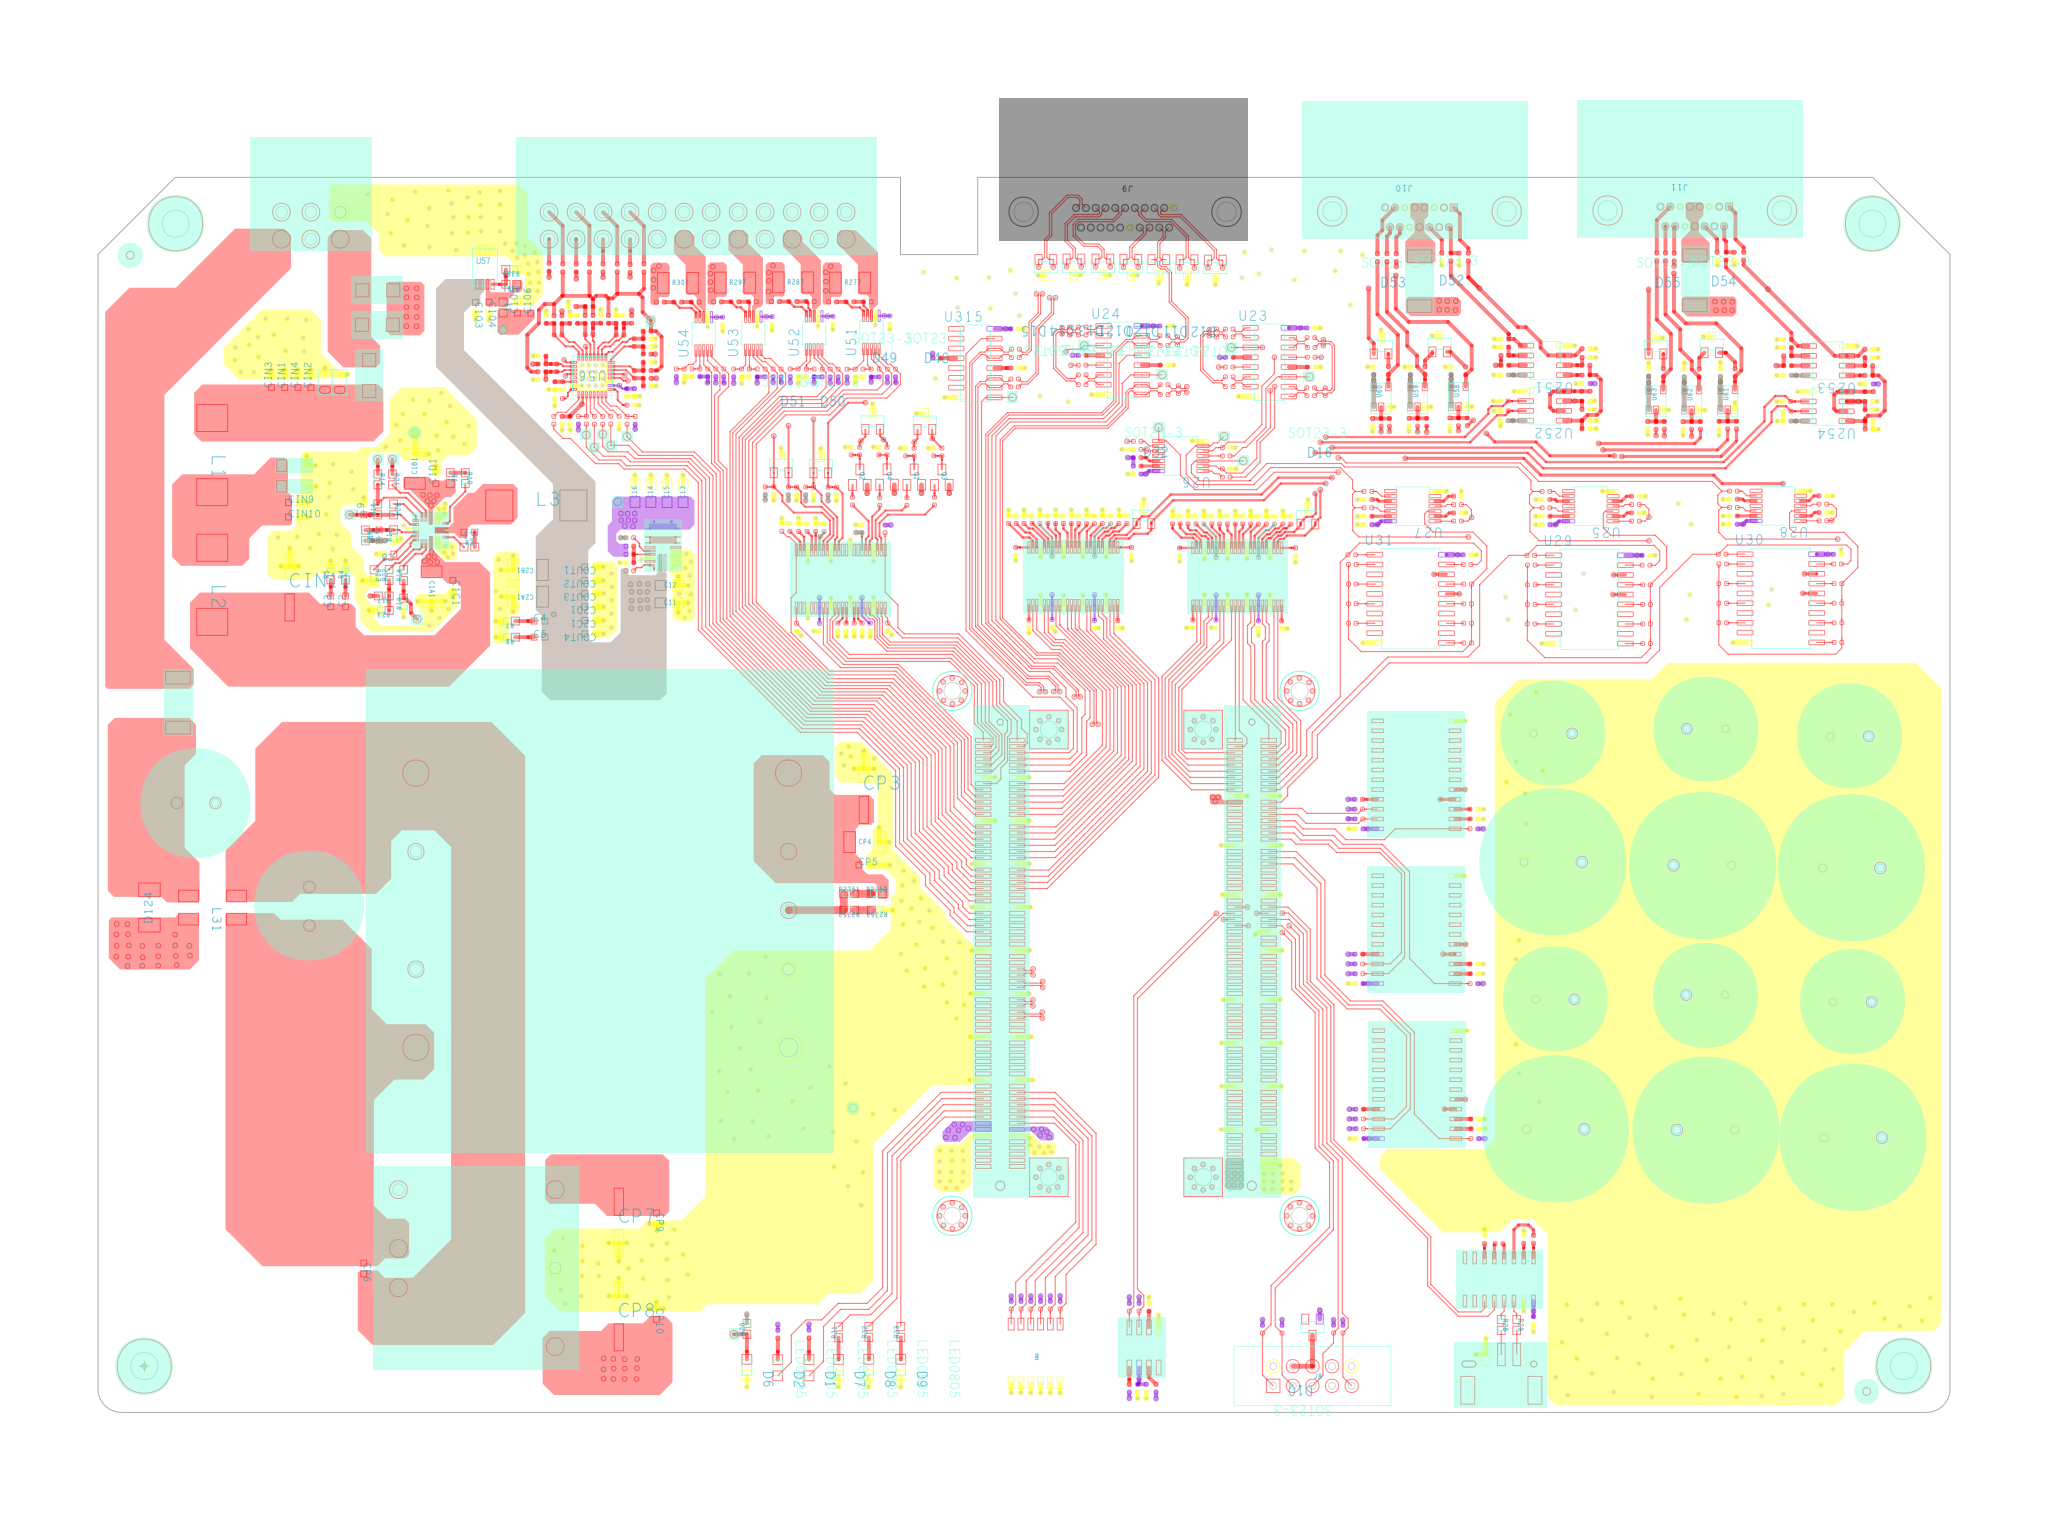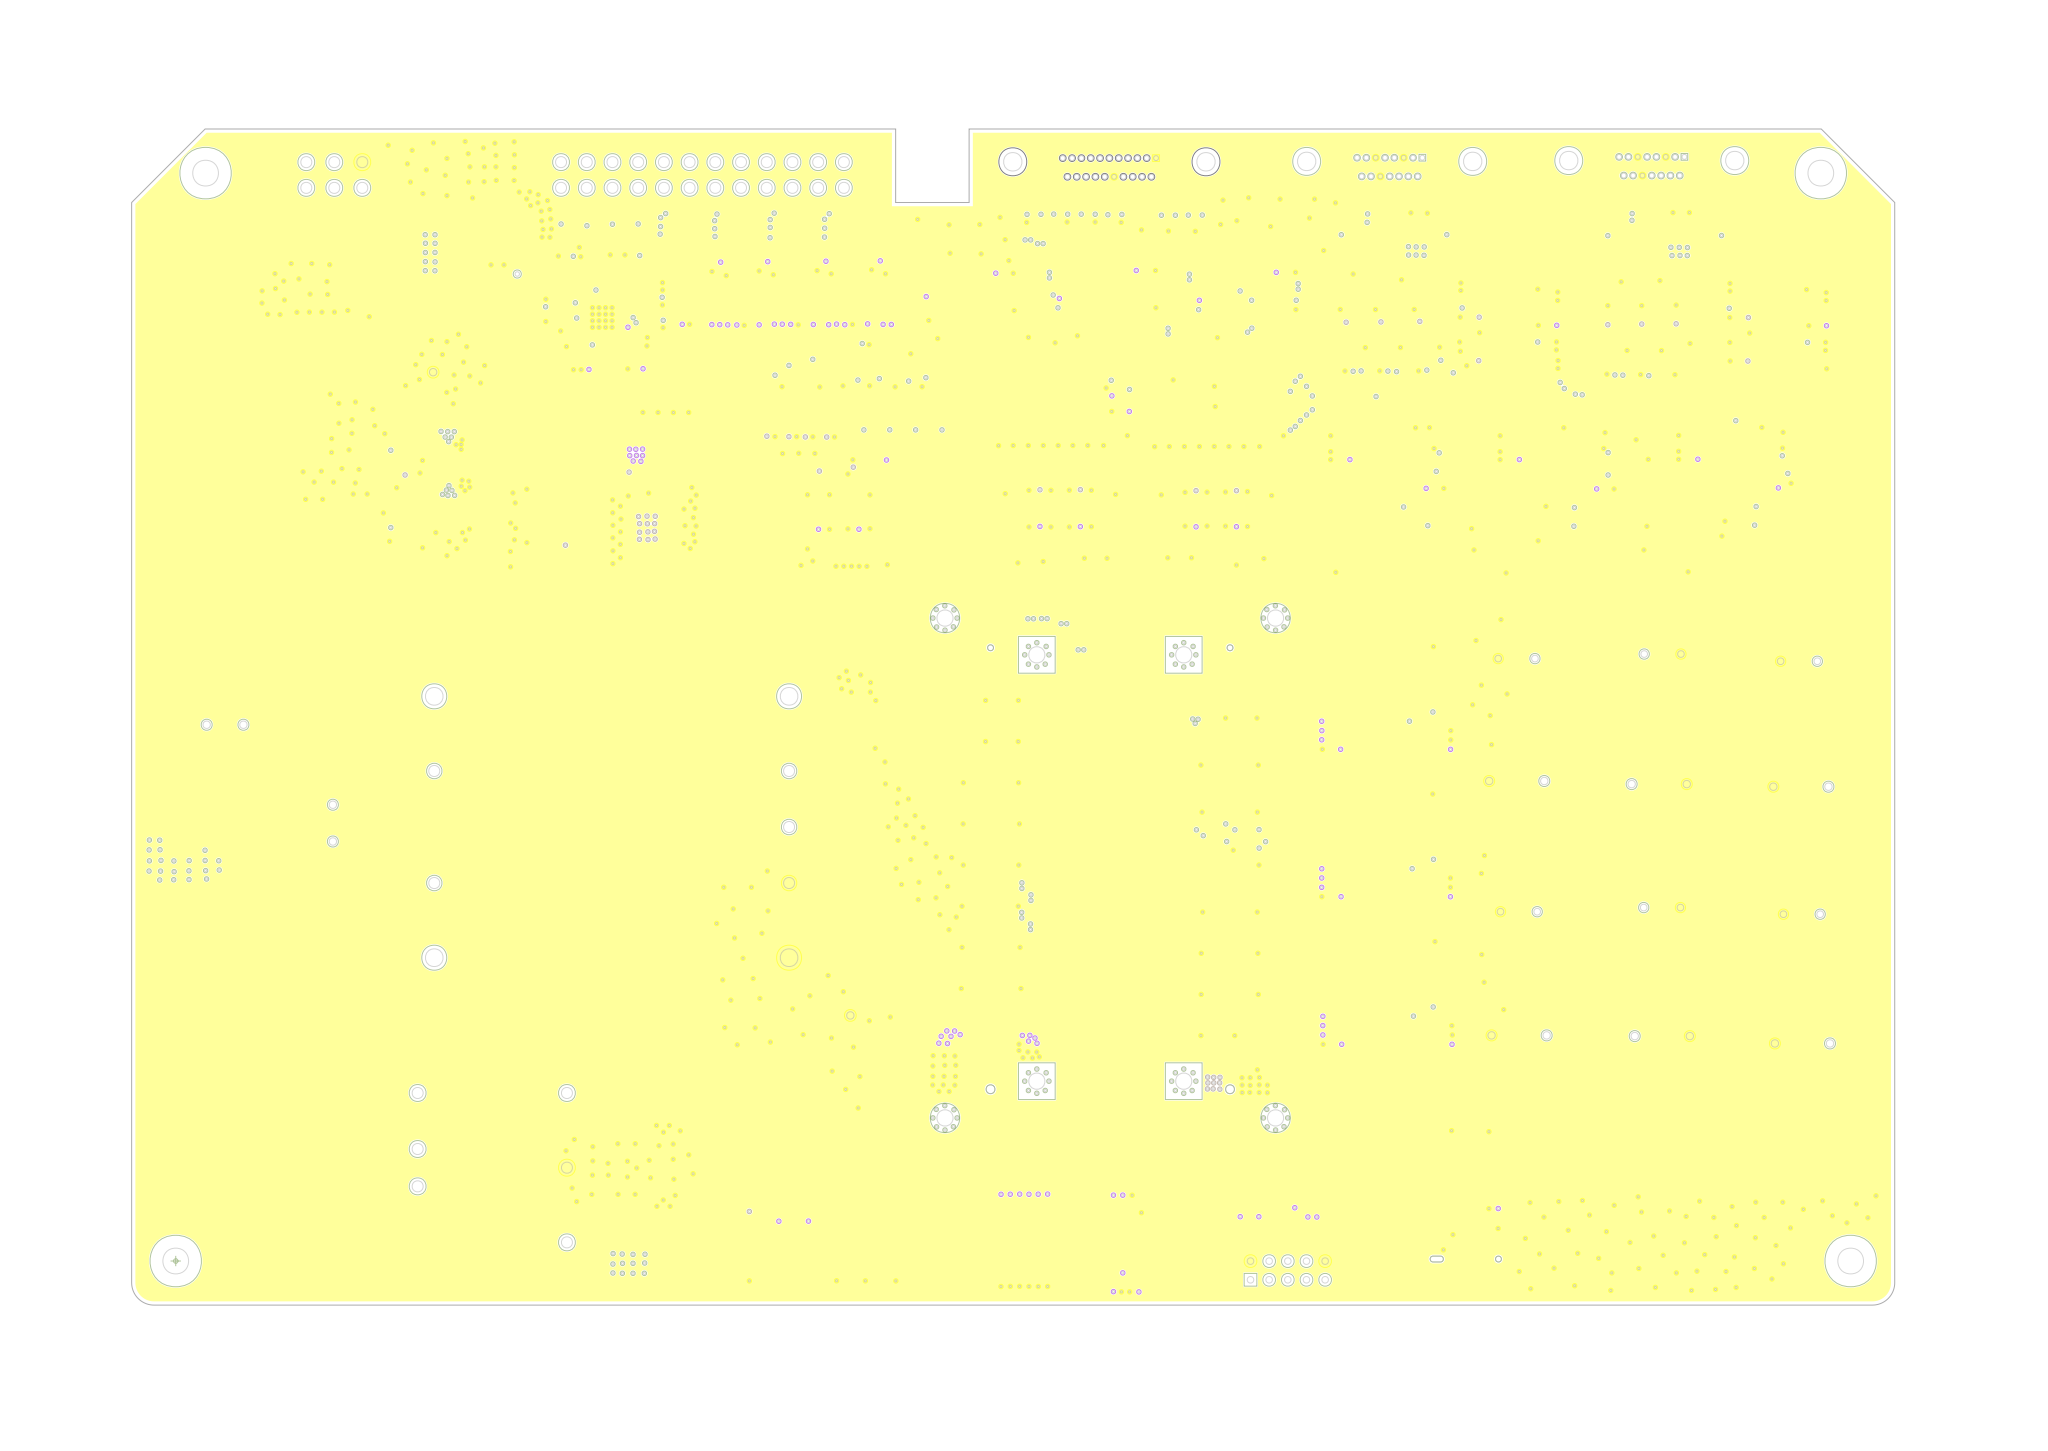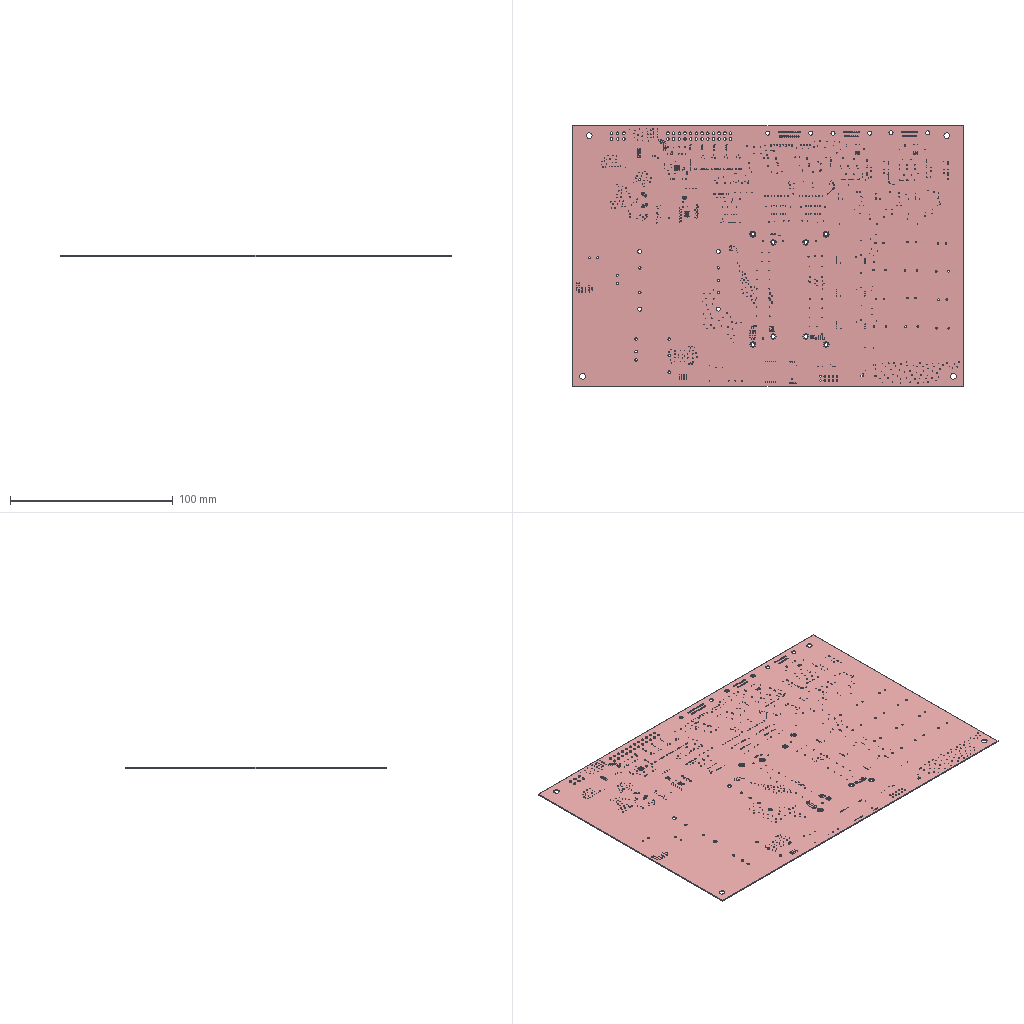Circuit board layout | Cadence Allegro | box 240 x 160 x 0.7 mm
Layer stack:
# Cadence Allegro layer stack of 2 (unit mm; from the constraint file cross-section; dielectric type: 0 not recorded (Allegro does not mark core vs prepreg), 3 surface material)
index,name,kind,layer,copper_thickness_mm,dielectric_type,dielectric_thickness_mm,dielectric_material,dielectric_constant
0,Top Surface,other,,,,,,
1,TOP,copper,TOP,0.0305,,,,
2,Dielectric1,dielectric,,,0,0.2032,FR-4,4.5
3,GND,copper,GND,0.0305,,,,
4,Dielectric2,dielectric,,,0,0.2032,FR-4,4.5
5,POWER,copper,POWER,0.0305,,,,
6,Dielectric3,dielectric,,,0,0.2032,FR-4,4.5
7,BOTTOM,copper,BOTTOM,0.0305,,,,
8,Bottom Surface,other,,,,,,
# drill layer pairs: low layer,high layer
drill_pair,TOP,BOTTOM
Part placement, first 399 of 635 lines:
REFDES,COMP_VALUE,SYM_NAME,SYM_X,SYM_Y,SYM_ROTATE,SYM_MIRROR
C1A1,CAP/1210,1210,1465.434,3976.499,270.000,NO
C1B1,CAP/1210,1210,1380.195,4577.161,90.000,NO
C1C1,CAP/0603,0603C,1574.039,4007.160,270.000,NO
C1D1,CAP/0603,0603C,1487.361,4501.515,90.000,NO
C2A1,CAP/1210,1210,1956.818,3924.329,180.000,NO
C2B1,CAP/1210,1210,1956.563,4060.550,180.000,NO
C2C1,CAP/0603,0603C,2303.126,3803.649,180.000,NO
C2D1,CAP/0603,0603C,2302.581,3873.143,180.000,NO
C1,CAP/0603,0603C,1685.688,4253.305,180.000,NO
C2,CAP/0603,0603C,1026.168,3873.029,90.000,NO
C3,CAP/0603,0603C,951.260,3873.232,90.000,NO
C4,CAP/0603,0603C,1988.129,3800.034,0.000,NO
C5,CAP/0603,0603C,1988.529,3717.881,0.000,NO
C6,CAP/0603,0603C,1198.333,4209.964,90.000,NO
C8,CAP/0603,0603C,1272.886,4141.786,180.000,NO
C9,CAP/0603,0603C,1120.158,4341.894,90.000,NO
C10,0.1uF/50V/10%/X7R/C0402,0402,7086.964,232.518,270.000,NO
C11,22uF/10V/10%/X5R/C0805,0805,2678.524,3892.734,0.000,NO
C12,22uF/10V/10%/X5R/C0805,0805,2678.800,3981.695,0.000,NO
C13,22uF/10V/10%/X5R/C0805,0805,2748.943,4451.876,90.000,NO
C14,22uF/10V/10%/X5R/C0805,0805,2584.754,4452.487,90.000,NO
C15,22uF/10V/10%/X5R/C0805,0805,2666.955,4451.762,90.000,NO
C16,22uF/10V/10%/X5R/C0805,0805,2503.522,4452.376,90.000,NO
C17,0.1uF/50V/10%/X7R/C0402,0402,7087.489,646.639,90.000,NO
C18,0.1uF/50V/10%/X7R/C0402,0402,6911.900,623.770,180.000,NO
C19,0.1uF/50V/10%/X7R/C0402,0402,7037.723,646.294,90.000,NO
C20,0.1uF/50V/10%/X7R/C0402,0402,6837.628,643.975,270.000,NO
C21,39pF/6.3V/5%/NP0/C0402,0402,2477.325,4140.263,180.000,NO
C22,1uF/16V/10%/X5R/C0402,0402,5068.182,-112.036,90.000,NO
C23,0.1uF/50V/10%/X7R/C0402,0402,5112.076,-112.284,90.000,NO
C24,0.1uF/50V/10%/X7R/C0402,0402,5125.671,299.907,90.000,NO
C25,0.1uF/50V/10%/X7R/C0402,0402,5951.524,5295.247,0.000,NO
C26,0.1uF/50V/10%/X7R/C0402,0402,5201.208,5305.263,0.000,NO
C27,0.1uF/50V/10%/X7R/C0402,0402,5065.955,4550.156,180.000,NO
C28,0.1uF/50V/10%/X7R/C0402,0402,7151.111,4291.950,180.000,NO
C29,0.1uF/50V/10%/X7R/C0402,0402,6242.994,4291.949,180.000,NO
C30,0.1uF/50V/10%/X7R/C0402,0402,8107.698,4293.779,180.000,NO
C31,0.1uF/50V/10%/X7R/C0402,0402,7660.842,4134.982,0.000,NO
C32,0.1uF/50V/10%/X7R/C0402,0402,6748.206,4138.240,0.000,NO
C33,0.1uF/50V/10%/X7R/C0402,0402,8637.483,4140.732,0.000,NO
C43,0.1uF/50V/10%/X7R/C0402,0402,6198.221,2740.667,0.000,NO
C45,0.1uF/50V/10%/X7R/C0402,0402,6198.573,1951.247,0.000,NO
C47,0.1uF/50V/10%/X7R/C0402,0402,6202.397,1160.643,0.000,NO
C49,0.1uF/50V/10%/X7R/C0402,0402,5766.891,4314.271,270.000,NO
C50,0.1uF/50V/10%/X7R/C0402,0402,5405.535,4315.049,270.000,NO
C51,0.1uF/50V/10%/X7R/C0402,0402,5467.835,3786.199,90.000,NO
C52,0.1uF/50V/10%/X7R/C0402,0402,5684.300,3781.656,90.000,NO
C57,0.1uF/50V/10%/X7R/C0402,0402,4930.365,4316.603,270.000,NO
C58,0.1uF/50V/10%/X7R/C0402,0402,4569.009,4317.381,270.000,NO
C59,0.1uF/50V/10%/X7R/C0402,0402,4847.774,3783.988,90.000,NO
C60,0.1uF/50V/10%/X7R/C0402,0402,4631.309,3788.531,90.000,NO
C65,0.1uF/50V/10%/X7R/C0402,0402,3803.741,5336.921,270.000,NO
C66,0.1uF/50V/10%/X7R/C0402,0402,3600.367,5428.470,0.000,NO
C67,0.1uF/50V/10%/X7R/C0402,0402,3512.888,5334.683,270.000,NO
C68,0.1uF/50V/10%/X7R/C0402,0402,3308.799,5429.878,0.000,NO
C69,0.1uF/50V/10%/X7R/C0402,0402,3202.484,5333.158,270.000,NO
C70,0.1uF/50V/10%/X7R/C0402,0402,3013.011,5428.470,0.000,NO
C71,0.1uF/50V/10%/X7R/C0402,0402,2950.344,5330.569,270.000,NO
C72,0.1uF/50V/10%/X7R/C0402,0402,2721.447,5427.062,0.000,NO
C73,0.1uF/50V/10%/X7R/C0402,0402,3661.662,4271.536,270.000,NO
C74,0.1uF/50V/10%/X7R/C0402,0402,3468.284,4276.953,270.000,NO
C75,0.1uF/50V/10%/X7R/C0402,0402,3444.743,3768.881,90.000,NO
C76,0.1uF/50V/10%/X7R/C0402,0402,3704.099,3770.174,90.000,NO
C77,10nF/50V/10%/X7R/C0402,0402,2565.299,4998.784,0.000,NO
C78,0.1uF/50V/10%/X7R/C0402,0402,2499.479,5058.201,90.000,NO
C79,10nF/50V/10%/X7R/C0402,0402,2565.078,5120.566,0.000,NO
C80,0.1uF/50V/10%/X7R/C0402,0402,2172.777,4824.301,270.000,NO
C81,1uF/50V/10%/X7R/C0402,0402,2131.567,4824.026,270.000,NO
C82,0.1uF/50V/10%/X7R/C0402,0402,2135.380,5001.091,270.000,NO
C83,1uF/50V/10%/X7R/C0402,0402,2094.388,5000.930,270.000,NO
C84,10nF/50V/10%/X7R/C0402,0402,2565.304,5200.458,0.000,NO
C85,0.1uF/50V/10%/X7R/C0402,0402,2497.547,5220.439,90.000,NO
C86,10nF/50V/10%/X7R/C0402,0402,2565.244,5240.239,0.000,NO
C87,0.1uF/50V/10%/X7R/C0402,0402,2113.766,4934.760,180.000,NO
C88,0.1uF/50V/10%/X7R/C0402,0402,2481.600,4901.211,0.000,NO
C89,0.1uF/50V/10%/X7R/C0402,0402,2460.040,4965.609,270.000,NO
C90,1uF/50V/10%/X7R/C0402,0402,2501.018,4966.074,270.000,NO
C91,10nF/50V/10%/X7R/C0402,0402,2446.425,5338.568,90.000,NO
C92,0.1uF/50V/10%/X7R/C0402,0402,2426.964,5258.168,180.000,NO
C93,10nF/50V/10%/X7R/C0402,0402,2407.207,5338.788,90.000,NO
C94,10nF/50V/10%/X7R/C0402,0402,2170.563,5338.047,90.000,NO
C95,0.1uF/50V/10%/X7R/C0402,0402,2110.730,5259.289,180.000,NO
C96,10nF/50V/10%/X7R/C0402,0402,2050.496,5337.941,90.000,NO
C99,10nF/50V/10%/X7R/C0402,0402,2029.187,5151.499,180.000,NO
C100,0.1uF/50V/10%/X7R/C0402,0402,2105.630,5091.446,270.000,NO
C101,10nF/50V/10%/X7R/C0402,0402,2028.852,5031.675,180.000,NO
C102,10nF/50V/10%/X7R/C0402,0402,2328.741,5338.869,90.000,NO
C103,1uF/25V/10%/X7R/C0603,0603C,1689.774,5424.503,270.000,NO
C104,1uF/25V/10%/X7R/C0603,0603C,1758.999,5426.586,270.000,NO
C105,10uF/10V/10%/X5R/C0603,0603C,1903.767,5370.918,90.000,NO
C106,0.1uF/50V/10%/X7R/C0603,0603C,1971.932,5370.859,90.000,NO
C107,0.1uF/50V/10%/X7R/C0402,0402,2269.120,5260.505,180.000,NO
C108,10nF/50V/10%/X7R/C0402,0402,2209.392,5338.368,90.000,NO
C109,0.1uF/50V/10%/X7R/C0402,0402,6666.908,5076.812,90.000,NO
C110,0.1uF/50V/10%/X7R/C0402,0402,6459.364,5076.456,90.000,NO
C111,0.1uF/50V/10%/X7R/C0402,0402,6272.476,5076.812,90.000,NO
C112,0.1uF/50V/10%/X7R/C0402,0402,8041.056,5066.436,90.000,NO
C113,0.1uF/50V/10%/X7R/C0402,0402,7674.891,5068.624,90.000,NO
C114,0.1uF/50V/10%/X7R/C0402,0402,7856.584,5065.004,90.000,NO
C795,0.1uF/50V/10%/X7R/C0402,0402,4439.984,5290.400,0.000,NO
C917,0.1uF/50V/10%/X7R/C0402,0402,6938.342,4822.335,180.000,NO
C918,2pF/50V/10%/X7R/C0402,0402,7354.384,4879.743,0.000,NO
C919,2pF/50V/10%/X7R/C0402,0402,7354.506,4822.784,0.000,NO
C920,0.1uF/50V/10%/X7R/C0402,0402,6940.936,5055.205,180.000,NO
C921,0.1uF/50V/10%/X7R/C0402,0402,8380.946,4820.319,180.000,NO
C922,0.1uF/50V/10%/X7R/C0402,0402,8383.540,5053.189,180.000,NO
C923,2pF/50V/10%/X7R/C0402,0402,8798.657,4877.394,0.000,NO
C924,2pF/50V/10%/X7R/C0402,0402,8799.113,4820.770,0.000,NO
C1046,10nF/50V/10%/X7R/C0402,0402,3211.543,4465.163,270.000,NO
C1047,10nF/50V/10%/X7R/C0402,0402,3414.415,4463.847,270.000,NO
C1048,10nF/50V/10%/X7R/C0402,0402,3327.631,4464.259,270.000,NO
C1049,10nF/50V/10%/X7R/C0402,0402,3530.643,4463.387,270.000,NO
CIN1,CAP/0603,0603C,716.126,4991.435,90.000,NO
CIN2,CAP/0603,0603C,850.372,4991.198,90.000,NO
CIN3,CAP/0603,0603C,649.394,4992.058,90.000,NO
CIN4,CAP/0603,0603C,783.533,4991.640,90.000,NO
CIN5,CAP/0603,0805C,921.995,5018.653,90.000,NO
CIN6,CAP/0603,0805C,996.502,5018.307,90.000,NO
CIN7,CAP/0603,1206,764.212,4593.485,0.000,NO
CIN8,CAP/0603,1206,763.877,4487.170,0.000,NO
CIN9,CAP/0603,0603C,735.616,4404.734,0.000,NO
CIN10,CAP/0603,0603C,735.616,4330.834,0.000,NO
CIN11,CAP/ELECT/DIP/OD5.3P2.0,AP-SMD_BD6_3-L6_6-W6_6-LS7_21,741.556,3974.623,90.000,NO
CIN12,ECF1HM182M27OTPO,AP-SMD_BD18-L27-W6_6-LS7_21,7186.624,2570.942,270.000,NO
CIN13,ECF1JM331G20OTPO,AP-SMD_BD10-L20-W6_6-LS7_21,7185.868,3226.632,270.000,NO
CIN14,ECF1HM182M27OTPO,AP-SMD_BD18-L27-W6_6-LS7_21,7199.516,1208.500,270.000,NO
CIN15,ECF1JM331G20OTPO,AP-SMD_BD10-L20-W6_6-LS7_21,7198.096,1870.916,270.000,NO
CIN16,ECF1HM182M27OTPO,AP-SMD_BD18-L27-W6_6-LS7_21,7966.783,1204.718,90.000,NO
CIN17,ECF1JM331G20OTPO,AP-SMD_BD10-L20-W6_6-LS7_21,7965.623,1893.086,90.000,NO
CIN18,ECF1HM182M27OTPO,AP-SMD_BD18-L27-W6_6-LS7_21,7950.310,2554.419,90.000,NO
CIN19,ECF1JM331G20OTPO,AP-SMD_BD10-L20-W6_6-LS7_21,7968.307,3250.966,90.000,NO
CIN20,ECF1HM182M27OTPO,AP-SMD_BD18-L27-W6_6-LS7_21,8709.621,2540.420,270.000,NO
CIN21,ECF1JM331G20OTPO,AP-SMD_BD10-L20-W6_6-LS7_21,8699.345,3212.322,270.000,NO
CIN22,ECF1HM182M27OTPO,AP-SMD_BD18-L27-W6_6-LS7_21,8717.937,1165.386,270.000,NO
CIN23,ECF1JM331G20OTPO,AP-SMD_BD10-L20-W6_6-LS7_21,8714.565,1857.490,270.000,NO
COUT1,CAP/0603,0603C,2302.361,4076.388,180.000,NO
COUT2,CAP/0603,0603C,2302.286,4007.628,180.000,NO
COUT3,CAP/0603,0603C,2302.924,3940.616,180.000,NO
COUT4,CAP/0603,0603C,2303.728,3735.215,180.000,NO
CP1,CAP/ELECT/DIP/OD5.3P2.0,AP-SMD_BD12_5-L20,264.324,2872.264,0.000,NO
CP2,CAP/ELECT/DIP/OD5.3P2.0,AP-SMD_BD12_5-L20,842.187,2345.380,270.000,NO
CP3,CAP/ELECT/DIP/OD5.3P2.0,AP-SMD_BD6_3-L6_6-W6_6-LS7_21,3670.733,2941.914,90.000,NO
CP4,CAP/1210,1210,3673.410,2672.756,0.000,NO
CP5,CAP/0603,0603C,3645.741,2555.662,0.000,NO
CP6,CAP/0603,0603C,1119.792,525.680,270.000,NO
CP7,CAP/ELECT/DIP/OD5.3P2.0,AP-SMD_BD6_3-L6_6-W6_6-LS7_21,2420.880,733.340,90.000,NO
CP8,CAP/ELECT/DIP/OD5.3P2.0,AP-SMD_BD6_3-L6_6-W6_6-LS7_21,2420.880,252.164,90.000,NO
CP9,CAP/0603,0603C,2613.744,781.072,270.000,NO
CP10,CAP/0603,0603C,2612.768,293.072,270.000,NO
D1,LED_GREEN,LED0805,3391.153,-8.170,270.000,NO
D2,LED_GREEN,LED0805,3231.645,-8.055,270.000,NO
D3,SS34,DO-214AC,1147.161,5052.210,270.000,NO
D6,LED_GREEN,LED0805,3074.152,-6.494,270.000,NO
D7,LED_GREEN,LED0805,3541.603,-6.906,270.000,NO
D8,LED_GREEN,LED0805,3695.910,-6.451,270.000,NO
D9,LED_GREEN,LED0805,3859.228,-6.536,270.000,NO
D10,BAT54C,SOT23,5959.891,198.860,180.000,NO
D11,PESD5V0L2BT,SOT23,5319.914,5602.014,180.000,NO
D12,PESD5V0L2BT,SOT23,5464.066,5600.018,180.000,NO
D13,PESD5V0L2BT,SOT23,4890.281,5605.666,180.000,NO
D14,PESD5V0L2BT,SOT23,4742.737,5605.666,180.000,NO
D15,PESD5V0L2BT,SOT23,4599.667,5603.752,180.000,NO
D16,PESD5V0L2BT,SOT23,5936.588,4335.974,0.000,NO
D32,PESD5V0L2BT,SOT23,5100.062,4338.306,0.000,NO
D48,PESD5V0L2BT,SOT23,3982.229,4818.243,0.000,NO
D49,PESD5V0L2BT,SOT23,3715.947,4818.975,0.000,NO
D50,PESD5V0L2BT,SOT23,3451.439,4596.863,0.000,NO
D51,PESD5V0L2BT,SOT23,3249.068,4597.791,0.000,NO
D52,PESD5V0L2BT,SOT23,6608.828,5214.298,0.000,NO
D53,PESD5V0L2BT,SOT23,6310.029,5203.769,0.000,NO
D54,PESD5V0L2BT,SOT23,7996.840,5209.814,0.000,NO
D55,PESD5V0L2BT,SOT23,7712.440,5203.528,0.000,NO
D120,PESD5V0L2BT,SOT23,5175.702,5602.685,180.000,NO
D121,PESD5V0L2BT,SOT23,5033.114,5603.965,180.000,NO
D122,SS34,DO-214AC,1189.269,5311.224,0.000,NO
D123,SS34,DO-214AC,1191.063,5487.208,0.000,NO
D124,SM6T56AY,DO-214AA,26.179,2339.032,90.000,NO
E1,Inductor_BEAD,0603R,1830.290,5399.204,270.000,NO
E14,Inductor_BEAD,0603R,1882.173,5925.017,0.000,YES
E15,Inductor_BEAD,0603R,1882.536,5994.352,0.000,YES
E16,Inductor_BEAD,0603R,1882.028,5856.252,0.000,YES
E17,Inductor_BEAD,0603R,1881.520,5787.460,0.000,YES
F1,0451010.MRL 125V@10A 2512,2512,171.492,3383.936,270.000,NO
J1,D2_3,D2_3,4614.756,3246.749,180.000,NO
J2,D2_3,D2_3,5402.154,3246.749,180.000,NO
J3,D2_3,D2_3,5402.154,963.280,180.000,NO
J4,D2_3,D2_3,4614.756,963.280,180.000,NO
J7,BM03B-PASS,BM03B-PASS,6923.507,59.754,0.000,NO
J8,TC2050_IDC_FP1,JTAG-10,5759.948,-100.535,0.000,NO
J9,J30JA-21ZKW-J,J30JA-21ZKW-J,5003.698,5887.469,180.000,NO
J10,J30JA-15ZKW-J,J30JA-15ZKW-J,6505.872,5889.544,180.000,NO
J11,J30JA-15ZKW-J,J30JA-15ZKW-J,7910.384,5894.004,180.000,NO
JX1,5177984-6,5177983-6,4366.721,2105.016,90.000,NO
JX2,5177984-6,5177983-6,5650.185,2105.016,90.000,NO
L1,CKST1004-1uH/M-B,SMD_10X11,346.314,4646.925,270.000,NO
L2,CKST1004-4.7uH/M,SMD_10X11,346.216,3984.972,270.000,NO
L3,CKST1004-4.7uH/M,SMD_10X11,2000.176,4389.846,0.000,NO
L31,YLM1513-701T,SMD_7X6MM,348.247,2338.740,270.000,NO
P1,F83-S-3.5-24pin,F83-S-3_5-24PIN,2822.870,5747.949,180.000,NO
P2,F83-S-3.81-6pin,F83-S-3_81-6PIN,849.744,5747.796,180.000,NO
Q1,S8050,SOT-23,3927.779,4533.749,270.000,NO
Q2,S8050,SOT-23,3650.422,4533.537,270.000,NO
Q3,S8050,SOT-23,4068.992,4533.332,270.000,NO
Q4,S8050,SOT-23,3789.052,4534.430,270.000,NO
R1,1K/62.5mW/1%/R0402,0402,3391.000,163.952,90.000,NO
R2,1K/62.5mW/1%/R0402,0402,3232.228,162.889,90.000,NO
R3,0/62.5mW/1%/R0603,0603R,1658.428,4177.456,0.000,NO
R4,10/62.5mW/1%/R0603,0603R,1026.009,4037.430,90.000,NO
R5,10/62.5mW/1%/R0603,0603R,951.264,4037.890,90.000,NO
R6,100K/62.5mW/1%/R0603,0603R,1560.839,4529.069,270.000,NO
R7,10/62.5mW/1%/R0603,0603R,1865.289,3800.193,180.000,NO
R8,10/62.5mW/1%/R0603,0603R,1865.325,3717.964,180.000,NO
R9,100K/62.5mW/1%/R0603,0603R,1128.152,4237.129,270.000,NO
R10,10/62.5mW/1%/R0603,0603R,1637.704,4528.939,270.000,NO
R12,19.6K/62.5mW/1%/R0603,0603R,1271.488,4237.678,90.000,NO
R13,62K/62.5mW/1%/R0603,0603R,1172.144,4034.230,270.000,NO
R14,10/62.5mW/1%/R0603,0603R,1191.305,4522.327,270.000,NO
R16,100K/62.5mW/1%/R0603,0603R,1190.815,4369.467,90.000,NO
R17,10/62.5mW/1%/R0603,0603R,1221.396,3928.232,180.000,NO
R18,10/62.5mW/1%/R0603,0603R,1322.955,4033.851,90.000,NO
R19,51K/62.5mW/1%/R0603,0603R,1322.916,3889.450,90.000,NO
R20,10K/62.5mW/1%/R0603,0603R,3074.090,189.923,90.000,NO
R21,10/62.5mW/1%/R0603,0603R,1265.684,4522.258,270.000,NO
R22,10/62.5mW/1%/R0603,0603R,1248.944,4035.206,90.000,NO
R23,0/62.5mW/1%/R0603,0603R,1221.711,3854.492,180.000,NO
R24,10/62.5mW/1%/R0603,0603R,1271.829,4369.506,270.000,NO
R25,499K/62.5mW/1%/R0402,0402,2476.720,4225.317,0.000,NO
R26,100k/62.5mW/1%/R0402,0402,2476.831,4056.949,180.000,NO
R27,20K/62.5mW/1%/R0402,0402,2477.212,4182.388,0.000,NO
R28,10/62.5mW/1%/R0603,0603R,6923.022,209.802,270.000,NO
R29,10/62.5mW/1%/R0603,0603R,7001.660,210.715,270.000,NO
R30,4.42K/62.5mW/1%/R0402,0402,2477.244,4097.576,0.000,NO
R31,10K/62.5mW/1%/R0603,0603R,3541.781,172.441,90.000,NO
R32,10K/62.5mW/1%/R0603,0603R,3696.642,174.411,90.000,NO
R33,10K/62.5mW/1%/R0603,0603R,3859.751,174.562,90.000,NO
R34,10K/62.5mW/1%/R0402,0402,4422.937,310.839,270.000,NO
R35,10K/62.5mW/1%/R0402,0402,4472.476,310.950,270.000,NO
R36,10K/62.5mW/1%/R0402,0402,4522.917,310.520,270.000,NO
R37,10K/62.5mW/1%/R0402,0402,4572.645,310.513,270.000,NO
R38,10K/62.5mW/1%/R0402,0402,4622.134,310.953,270.000,NO
R39,10K/62.5mW/1%/R0402,0402,4672.740,310.678,270.000,NO
R40,4.7K/62.5mW/1%/R0402,0402,5704.804,188.504,270.000,NO
R41,4.7K/62.5mW/1%/R0402,0402,5804.612,188.432,270.000,NO
R42,4.7K/62.5mW/1%/R0402,0402,6067.480,189.176,270.000,NO
R43,4.7K/62.5mW/1%/R0402,0402,6115.248,188.844,270.000,NO
R44,4.7K/62.5mW/1%/R0402,0402,5161.812,-112.620,90.000,NO
R45,4.7K/62.5mW/1%/R0402,0402,5025.475,-113.306,90.000,NO
R46,4.7K/62.5mW/1%/R0402,0402,5025.425,300.205,270.000,NO
R47,4.7K/62.5mW/1%/R0402,0402,5075.349,300.222,270.000,NO
R48,22/62.5mW/1%/R0402,0402,5953.854,5095.751,0.000,NO
R49,0/62.5mW/1%/R0402,0402,5535.386,5249.841,0.000,NO
R50,0/62.5mW/1%/R0402,0402,5535.292,5288.963,0.000,NO
R51,22/62.5mW/1%/R0402,0402,5203.538,5105.767,0.000,NO
R52,0/62.5mW/1%/R0402,0402,5535.379,5045.522,0.000,NO
R53,0/62.5mW/1%/R0402,0402,4785.070,5259.857,0.000,NO
R54,0/62.5mW/1%/R0402,0402,4784.976,5298.979,0.000,NO
R55,0/62.5mW/1%/R0402,0402,5535.158,4995.824,0.000,NO
R56,0/62.5mW/1%/R0402,0402,4785.063,5055.538,0.000,NO
R57,0/62.5mW/1%/R0402,0402,5950.603,4989.357,180.000,NO
R58,0/62.5mW/1%/R0402,0402,4784.842,5005.840,0.000,NO
R59,10K/62.5mW/1%/R0402,0402,5535.949,5145.458,0.000,NO
R60,0/62.5mW/1%/R0402,0402,5951.166,4949.684,180.000,NO
R61,0/62.5mW/1%/R0402,0402,5953.217,5195.503,180.000,NO
R62,10K/62.5mW/1%/R0402,0402,4785.633,5155.474,0.000,NO
R63,0/62.5mW/1%/R0402,0402,5952.107,5245.526,180.000,NO
R64,0/62.5mW/1%/R0402,0402,5202.994,5005.686,180.000,NO
R65,0/62.5mW/1%/R0402,0402,5203.290,4955.649,180.000,NO
R66,0/62.5mW/1%/R0402,0402,5202.901,5205.519,180.000,NO
R67,0/62.5mW/1%/R0402,0402,5201.791,5255.542,180.000,NO
R68,0/62.5mW/1%/R0402,0402,5519.910,4534.523,180.000,NO
R69,0/62.5mW/1%/R0402,0402,7607.919,4309.953,180.000,NO
R70,0/62.5mW/1%/R0402,0402,7607.612,4394.296,180.000,NO
R71,1k/62.5mW/1%/R0402,0402,5519.800,4576.523,180.000,NO
R72,0/62.5mW/1%/R0402,0402,5519.831,4642.186,180.000,NO
R73,0/62.5mW/1%/R0402,0402,6699.802,4309.952,180.000,NO
R74,0/62.5mW/1%/R0402,0402,6699.495,4394.295,180.000,NO
R75,0/62.5mW/1%/R0402,0402,8564.506,4311.782,180.000,NO
R76,0/62.5mW/1%/R0402,0402,7607.809,4351.953,180.000,NO
R77,0/62.5mW/1%/R0402,0402,6699.692,4351.952,180.000,NO
R78,0/62.5mW/1%/R0402,0402,8564.199,4396.125,180.000,NO
R79,0/62.5mW/1%/R0402,0402,8564.396,4353.782,180.000,NO
R80,1k/62.5mW/1%/R0402,0402,5519.709,4684.753,180.000,NO
R81,0/62.5mW/1%/R0402,0402,7607.490,4436.863,180.000,NO
R82,0/62.5mW/1%/R0402,0402,6699.373,4436.862,180.000,NO
R83,0/62.5mW/1%/R0402,0402,8564.077,4438.692,180.000,NO
R84,0/62.5mW/1%/R0402,0402,5065.540,4717.116,0.000,NO
R85,0/62.5mW/1%/R0402,0402,7151.067,4461.202,0.000,NO
R86,0/62.5mW/1%/R0402,0402,6242.950,4461.201,0.000,NO
R87,0/62.5mW/1%/R0402,0402,8107.654,4463.031,0.000,NO
R88,1k/62.5mW/1%/R0402,0402,5065.702,4675.955,0.000,NO
R89,0/62.5mW/1%/R0402,0402,7151.229,4420.040,0.000,NO
R90,0/62.5mW/1%/R0402,0402,6243.112,4420.039,0.000,NO
R91,0/62.5mW/1%/R0402,0402,8107.816,4421.869,0.000,NO
R92,1k/62.5mW/1%/R0402,0402,5065.501,4633.754,0.000,NO
R93,0/62.5mW/1%/R0402,0402,7151.028,4377.840,0.000,NO
R94,0/62.5mW/1%/R0402,0402,6242.911,4377.839,0.000,NO
R95,0/62.5mW/1%/R0402,0402,8107.615,4379.669,0.000,NO
R96,1k/62.5mW/1%/R0402,0402,5065.662,4590.620,0.000,NO
R97,0/62.5mW/1%/R0402,0402,7151.189,4334.706,0.000,NO
R98,0/62.5mW/1%/R0402,0402,6243.072,4334.705,0.000,NO
R99,0/62.5mW/1%/R0402,0402,8107.776,4336.535,0.000,NO
R100,0/62.5mW/1%/R0402,0402,7076.219,4085.572,0.000,NO
R101,0/62.5mW/1%/R0402,0402,6163.583,4088.830,0.000,NO
R102,0/62.5mW/1%/R0402,0402,8052.860,4091.322,0.000,NO
R103,0/62.5mW/1%/R0402,0402,7076.141,3985.465,0.000,NO
R104,0/62.5mW/1%/R0402,0402,7075.987,3885.370,0.000,NO
R105,0/62.5mW/1%/R0402,0402,6163.505,3988.723,0.000,NO
R106,0/62.5mW/1%/R0402,0402,8052.628,3891.120,0.000,NO
R107,0/62.5mW/1%/R0402,0402,6163.217,3788.924,0.000,NO
R108,0/62.5mW/1%/R0402,0402,6163.351,3888.628,0.000,NO
R109,0/62.5mW/1%/R0402,0402,7075.853,3785.666,0.000,NO
R110,0/62.5mW/1%/R0402,0402,8052.782,3991.215,0.000,NO
R111,0/62.5mW/1%/R0402,0402,8052.494,3791.416,0.000,NO
R112,0/62.5mW/1%/R0402,0402,7664.139,3685.691,180.000,NO
R113,0/62.5mW/1%/R0402,0402,6751.503,3688.491,180.000,NO
R114,0/62.5mW/1%/R0402,0402,8640.780,3691.057,180.000,NO
R115,0/62.5mW/1%/R0402,0402,7664.395,3785.755,180.000,NO
R116,0/62.5mW/1%/R0402,0402,6751.759,3789.013,180.000,NO
R117,0/62.5mW/1%/R0402,0402,8641.036,3791.301,180.000,NO
R118,0/62.5mW/1%/R0402,0402,7663.976,3885.181,180.000,NO
R119,0/62.5mW/1%/R0402,0402,6751.340,3888.439,180.000,NO
R120,0/62.5mW/1%/R0402,0402,8640.719,3891.135,180.000,NO
R121,0/62.5mW/1%/R0402,0402,7664.109,3985.288,180.000,NO
R122,0/62.5mW/1%/R0402,0402,6751.473,3988.546,180.000,NO
R123,0/62.5mW/1%/R0402,0402,8640.750,3991.140,180.000,NO
R124,0/62.5mW/1%/R0402,0402,7661.573,4085.193,180.000,NO
R125,0/62.5mW/1%/R0402,0402,6748.937,4088.451,180.000,NO
R126,0/62.5mW/1%/R0402,0402,8638.214,4091.147,180.000,NO
R127,0/62.5mW/1%/R0402,0402,7073.447,4135.209,0.000,NO
R128,0/62.5mW/1%/R0402,0402,6160.811,4138.467,0.000,NO
R129,0/62.5mW/1%/R0402,0402,8050.088,4140.959,0.000,NO
R220,10K/62.5mW/1%/R0402,0402,6195.676,2890.858,0.000,NO
R221,10K/62.5mW/1%/R0402,0402,6784.445,2790.804,180.000,NO
R222,10K/62.5mW/1%/R0402,0402,6783.181,2840.724,180.000,NO
R226,10K/62.5mW/1%/R0402,0402,6783.382,2740.450,0.000,NO
R228,10K/62.5mW/1%/R0402,0402,6195.866,2840.911,180.000,NO
R230,10K/62.5mW/1%/R0402,0402,6197.177,2790.860,180.000,NO
R232,10K/62.5mW/1%/R0402,0402,6196.232,2101.029,0.000,NO
R233,10K/62.5mW/1%/R0402,0402,6784.797,2001.384,180.000,NO
R234,10K/62.5mW/1%/R0402,0402,6783.533,2051.304,180.000,NO
R238,10K/62.5mW/1%/R0402,0402,6783.734,1951.030,0.000,NO
R240,10K/62.5mW/1%/R0402,0402,6196.218,2051.491,180.000,NO
R242,10K/62.5mW/1%/R0402,0402,6197.529,2001.440,180.000,NO
R244,10K/62.5mW/1%/R0402,0402,6200.056,1310.425,0.000,NO
R245,10K/62.5mW/1%/R0402,0402,6788.621,1210.780,180.000,NO
R246,10K/62.5mW/1%/R0402,0402,6787.357,1260.700,180.000,NO
R250,10K/62.5mW/1%/R0402,0402,6787.558,1160.426,0.000,NO
R252,10K/62.5mW/1%/R0402,0402,6200.042,1260.887,180.000,NO
R254,10K/62.5mW/1%/R0402,0402,6201.353,1210.836,180.000,NO
R256,10K/62.5mW/1%/R0402,0402,5873.295,4153.848,90.000,NO
R257,10K/62.5mW/1%/R0402,0402,5802.647,3781.814,90.000,NO
R260,10K/62.5mW/1%/R0402,0402,5349.778,3786.077,90.000,NO
R261,10K/62.5mW/1%/R0402,0402,5281.920,4153.791,90.000,NO
R264,10K/62.5mW/1%/R0402,0402,5036.769,4156.180,90.000,NO
R265,10K/62.5mW/1%/R0402,0402,4966.121,3783.645,90.000,NO
R268,10K/62.5mW/1%/R0402,0402,4513.252,3786.574,90.000,NO
R269,10K/62.5mW/1%/R0402,0402,4445.394,4156.123,90.000,NO
R272,10k/62.5mW/1%/R0402,0402,3708.184,5065.307,90.000,NO
R273,10k/62.5mW/1%/R0402,0402,3585.632,5065.066,90.000,NO
R274,10k/62.5mW/1%/R0402,0402,3667.115,5065.378,270.000,NO
R275,10k/62.5mW/1%/R0402,0402,3626.682,5065.003,270.000,NO
R276,4.7R/62.5mW/1%/R0402,0402,3511.418,5428.261,180.000,NO
R277,20m/0.5W/0.01%/R1210,1210,3601.154,5526.368,0.000,NO
R278,4.7R/62.5mW/1%/R0402,0402,3689.497,5428.671,0.000,NO
R279,10k/62.5mW/1%/R0402,0402,3749.596,5065.383,270.000,NO
R280,10k/62.5mW/1%/R0402,0402,3832.528,5065.469,270.000,NO
R281,10k/62.5mW/1%/R0402,0402,3790.861,5065.465,270.000,NO
R282,10k/62.5mW/1%/R0402,0402,3416.950,5066.304,90.000,NO
R283,10k/62.5mW/1%/R0402,0402,3295.733,5066.229,90.000,NO
R284,10k/62.5mW/1%/R0402,0402,3377.550,5066.375,270.000,NO
R285,10k/62.5mW/1%/R0402,0402,3336.116,5066.500,270.000,NO
R286,4.7R/62.5mW/1%/R0402,0402,3219.850,5429.669,180.000,NO
R287,20m/0.5W/0.01%/R1210,1210,3309.586,5527.776,0.000,NO
R288,4.7R/62.5mW/1%/R0402,0402,3397.929,5430.079,0.000,NO
R289,10k/62.5mW/1%/R0402,0402,3458.696,5065.212,270.000,NO
R290,10k/62.5mW/1%/R0402,0402,3539.680,5065.294,270.000,NO
R291,10k/62.5mW/1%/R0402,0402,3499.239,5065.298,270.000,NO
R292,10k/62.5mW/1%/R0402,0402,3126.784,5065.728,90.000,NO
R293,10k/62.5mW/1%/R0402,0402,3007.019,5065.803,90.000,NO
R294,10k/62.5mW/1%/R0402,0402,3087.062,5065.665,270.000,NO
R295,10k/62.5mW/1%/R0402,0402,3046.723,5065.874,270.000,NO
R296,4.7R/62.5mW/1%/R0402,0402,2924.062,5428.261,180.000,NO
R297,20m/0.5W/0.01%/R1210,1210,3013.798,5526.368,0.000,NO
R298,4.7R/62.5mW/1%/R0402,0402,3102.141,5428.671,0.000,NO
R299,10k/62.5mW/1%/R0402,0402,3167.587,5065.712,270.000,NO
R300,10k/62.5mW/1%/R0402,0402,3248.571,5065.794,270.000,NO
R301,10k/62.5mW/1%/R0402,0402,3208.130,5065.798,270.000,NO
R302,10k/62.5mW/1%/R0402,0402,2834.206,5066.726,90.000,NO
R303,10k/62.5mW/1%/R0402,0402,2714.441,5066.801,90.000,NO
R304,10k/62.5mW/1%/R0402,0402,2794.484,5066.663,270.000,NO
R305,10k/62.5mW/1%/R0402,0402,2754.145,5066.872,270.000,NO
R306,4.7R/62.5mW/1%/R0402,0402,2632.498,5426.853,180.000,NO
R307,20m/0.5W/0.01%/R1210,1210,2722.234,5524.960,0.000,NO
R308,4.7R/62.5mW/1%/R0402,0402,2810.577,5427.263,0.000,NO
R309,10k/62.5mW/1%/R0402,0402,2875.009,5066.710,270.000,NO
R310,10k/62.5mW/1%/R0402,0402,2955.993,5066.792,270.000,NO
R311,10k/62.5mW/1%/R0402,0402,2915.552,5066.796,270.000,NO
R312,22/62.5mW/0.1%/R0402,0402,4069.280,4662.423,270.000,NO
Pad and via stacks, first 108 of 133 lines:
# Allegro (Cadence) via spans and padstacks; design units: ("mils" 3 1000)
# via spans: padstack,start_layer,end_layer,net_example,count
VIA12_24,ETCH/TOP,ETCH/BOTTOM,32VINGND,1057
# Allegro padstack definitions: name,start_layer,end_layer,drill,plating,holeType,type
2020B,"ETCH/TOP","ETCH/TOP",0.0,"PLATED","none","smd"
SMD_R551X500P0S40,"ETCH/TOP","ETCH/TOP",0.0,"PLATED","none","smd"
PSM_065X081R,"ETCH/TOP","ETCH/TOP",0.0,"PLATED","none","smd"
SMD50_50,"ETCH/TOP","ETCH/TOP",0.0,"PLATED","none","smd"
SMD200X50,"ETCH/TOP","ETCH/TOP",0.0,"PLATED","none","smd"
R75X85,"ETCH/TOP","ETCH/TOP",0.0,"NON_PLATED","none","smd"
RE55X40,"ETCH/TOP","ETCH/TOP",0.0,"NON_PLATED","none","smd"
SMD_R591X1063P0S40,"ETCH/TOP","ETCH/TOP",0.0,"PLATED","none","smd"
Y10,"ETCH/TOP","ETCH/TOP",0.0,"NON_PLATED","none","smd"
R61X15,"ETCH/TOP","ETCH/TOP",0.0,"NON_PLATED","none","smd"
SMD_S50P0S40,"ETCH/TOP","ETCH/TOP",0.0,"PLATED","none","smd"
SMD_R510X80P0S0,"ETCH/TOP","ETCH/TOP",0.0,"PLATED","none","smd"
SMD_R810X100P0S0,"ETCH/TOP","ETCH/TOP",0.0,"PLATED","none","smd"
R150_30_K,"ETCH/TOP","ETCH/TOP",0.0,"NON_PLATED","none","smd"
RX148Y148D0T,"ETCH/TOP","ETCH/TOP",0.0,"PLATED","none","smd"
RX10Y32D0T,"ETCH/TOP","ETCH/TOP",0.0,"PLATED","none","smd"
SMD36_50,"ETCH/TOP","ETCH/TOP",0.0,"PLATED","none","smd"
PSM_091S_PM,"ETCH/TOP","ETCH/TOP",0.0,"NON_PLATED","none","smd"
R105_100,"ETCH/TOP","ETCH/TOP",0.0,"PLATED","none","smd"
BGA10_SMD0X619,"ETCH/TOP","ETCH/TOP",0.0,"NON_PLATED","none","smd"
O0R9X1R4,"ETCH/TOP","ETCH/TOP",0.0,"NON_PLATED","none","smd"
R127X152,"ETCH/TOP","ETCH/TOP",0.0,"NON_PLATED","none","smd"
SMD_R1378X472P0S20,"ETCH/TOP","ETCH/TOP",0.0,"PLATED","none","smd"
SMD_R600X300P0S20,"ETCH/TOP","ETCH/TOP",0.0,"PLATED","none","smd"
SMD_R1378X1575P0S20,"ETCH/TOP","ETCH/TOP",0.0,"PLATED","none","smd"
RX43Y10D0T,"ETCH/TOP","ETCH/TOP",0.0,"PLATED","none","smd"
RX59Y10D0T,"ETCH/TOP","ETCH/TOP",0.0,"PLATED","none","smd"
RX5Y5D0T,"ETCH/TOP","ETCH/TOP",0.0,"PLATED","none","smd"
RX28Y10D0T,"ETCH/TOP","ETCH/TOP",0.0,"PLATED","none","smd"
SMD_S300P0S10,"ETCH/TOP","ETCH/TOP",0.0,"PLATED","none","smd"
Y3_MARK,"ETCH/TOP","ETCH/TOP",0.0,"PLATED","none","smd"
F45,"ETCH/TOP","ETCH/TOP",0.0,"PLATED","none","smd"
R91X127,"ETCH/TOP","ETCH/TOP",0.0,"NON_PLATED","none","smd"
S91,"ETCH/TOP","ETCH/TOP",0.0,"NON_PLATED","none","smd"
R127X120,"ETCH/TOP","ETCH/TOP",0.0,"NON_PLATED","none","smd"
R40X36,"ETCH/TOP","ETCH/TOP",0.0,"PLATED","none","smd"
R127X121,"ETCH/TOP","ETCH/TOP",0.0,"PLATED","none","smd"
R88X76,"ETCH/TOP","ETCH/TOP",0.0,"PLATED","none","smd"
R60X20,"ETCH/TOP","ETCH/TOP",0.0,"PLATED","none","smd"
R120X70,"ETCH/TOP","ETCH/TOP",0.0,"PLATED","none","smd"
R50X32,"ETCH/TOP","ETCH/TOP",0.0,"PLATED","none","smd"
S437,"ETCH/TOP","ETCH/TOP",0.0,"PLATED","none","smd"
Y4,"ETCH/TOP","ETCH/TOP",0.0,"PLATED","none","smd"
SMD0_45R,"ETCH/TOP","ETCH/TOP",0.0,"PLATED","none","smd"
R85X65,"ETCH/TOP","ETCH/TOP",0.0,"PLATED","none","smd"
Y50,"ETCH/TOP","ETCH/TOP",0.0,"PLATED","none","smd"
RE43_31X19_68,"ETCH/TOP","ETCH/TOP",0.0,"PLATED","none","smd"
RE134X170,"ETCH/TOP","ETCH/TOP",0.0,"PLATED","none","smd"
SMD_R98X276P0S30,"ETCH/TOP","ETCH/TOP",0.0,"PLATED","none","smd"
SMD_R98X433P0S30,"ETCH/TOP","ETCH/TOP",0.0,"PLATED","none","smd"
SMD_R98X276P0S10,"ETCH/TOP","ETCH/TOP",0.0,"PLATED","none","smd"
SMD_R98X433P0S10,"ETCH/TOP","ETCH/TOP",0.0,"PLATED","none","smd"
SMD_R236X669P0S40,"ETCH/TOP","ETCH/TOP",0.0,"PLATED","none","smd"
SMD_R236X669P0S30,"ETCH/TOP","ETCH/TOP",0.0,"PLATED","none","smd"
SMD_R98X433S30,"ETCH/TOP","ETCH/TOP",0.0,"PLATED","none","smd"
C12_6,"ETCH/TOP","ETCH/TOP",0.0,"PLATED","none","smd"
R80X25,"ETCH/TOP","ETCH/TOP",0.0,"PLATED","none","smd"
SMD10_61,"ETCH/TOP","ETCH/TOP",0.0,"PLATED","none","smd"
R29_92X50,"ETCH/TOP","ETCH/TOP",0.0,"PLATED","none","smd"
S_R197T60D5M197_60P197_60,"ETCH/TOP","ETCH/TOP",0.0,"PLATED","none","smd"
R36X18,"ETCH/TOP","ETCH/TOP",0.0,"PLATED","none","smd"
R29X10,"ETCH/TOP","ETCH/TOP",0.0,"PLATED","none","smd"
S17,"ETCH/TOP","ETCH/TOP",0.0,"NON_PLATED","none","smd"
R165X317,"ETCH/TOP","ETCH/TOP",0.0,"NON_PLATED","none","smd"
RE39_37X27_56,"ETCH/TOP","ETCH/TOP",0.0,"NON_PLATED","none","smd"
PAD18,"ETCH/TOP","ETCH/TOP",0.0,"NON_PLATED","none","smd"
R45X150,"ETCH/TOP","ETCH/TOP",0.0,"NON_PLATED","none","smd"
S_R206T60D2M206_60P206_60,"ETCH/TOP","ETCH/TOP",0.0,"PLATED","none","smd"
S_R197T60D2M197_60P197_60,"ETCH/TOP","ETCH/TOP",0.0,"PLATED","none","smd"
S_R157T41D2M157_41P157_41,"ETCH/TOP","ETCH/TOP",0.0,"PLATED","none","smd"
S_R147T28D2M147_28P147_28,"ETCH/TOP","ETCH/TOP",0.0,"PLATED","none","smd"
SMD_R1024X591P0S40,"ETCH/TOP","ETCH/TOP",0.0,"PLATED","none","smd"
SMD70X110,"ETCH/TOP","ETCH/TOP",0.0,"PLATED","none","smd"
Y24,"ETCH/TOP","ETCH/BOTTOM",51.181,"PLATED","circle_drill","through"
C68_11D35,"ETCH/TOP","ETCH/BOTTOM",35.039,"PLATED","circle_drill","through"
SQ68_11D35,"ETCH/TOP","ETCH/BOTTOM",35.039,"PLATED","circle_drill","through"
C130D130N,"ETCH/TOP","ETCH/BOTTOM",129.921,"NON_PLATED","circle_drill","through"
C98D70_87,"ETCH/TOP","ETCH/BOTTOM",70.87,"PLATED","circle_drill","through"
C70_87D51_18,"ETCH/TOP","ETCH/BOTTOM",51.181,"PLATED","circle_drill","through"
C60D40,"ETCH/TOP","ETCH/BOTTOM",40.0,"PLATED","circle_drill","through"
Y0_80,"ETCH/TOP","ETCH/BOTTOM",31.496,"NON_PLATED","circle_drill","through"
Y0_120,"ETCH/TOP","ETCH/BOTTOM",47.244,"NON_PLATED","circle_drill","through"
Y60,"ETCH/TOP","ETCH/BOTTOM",123.622,"PLATED","circle_drill","through"
Y0_0_6,"ETCH/TOP","ETCH/BOTTOM",23.622,"PLATED","circle_drill","through"
Y1000,"ETCH/TOP","ETCH/BOTTOM",39.37,"PLATED","circle_drill","through"
Y3000,"ETCH/TOP","ETCH/BOTTOM",78.74,"PLATED","circle_drill","through"
VIA24D12,"ETCH/TOP","ETCH/BOTTOM",12.0,"PLATED","circle_drill","through"
Y4_6,"ETCH/TOP","ETCH/BOTTOM",86.614,"PLATED","circle_drill","through"
F152,"ETCH/TOP","ETCH/BOTTOM",40.0,"PLATED","circle_drill","through"
F15,"ETCH/TOP","ETCH/BOTTOM",40.0,"PLATED","circle_drill","through"
Y150_1,"ETCH/TOP","ETCH/BOTTOM",59.055,"PLATED","circle_drill","through"
D3,"ETCH/TOP","ETCH/BOTTOM",118.11,"NON_PLATED","circle_drill","through"
Y328,"ETCH/TOP","ETCH/BOTTOM",129.134,"NON_PLATED","circle_drill","through"
Y300_1,"ETCH/TOP","ETCH/BOTTOM",125.0,"NON_PLATED","circle_drill","through"
Y4_5,"ETCH/TOP","ETCH/BOTTOM",86.614,"PLATED","circle_drill","through"
VIA_D10C020,"ETCH/TOP","ETCH/BOTTOM",10.0,"PLATED","circle_drill","through"
EX63Y63D43P,"ETCH/TOP","ETCH/BOTTOM",43.0,"PLATED","circle_drill","through"
EX83Y83D63P,"ETCH/TOP","ETCH/BOTTOM",63.0,"PLATED","circle_drill","through"
T18X9,"ETCH/TOP","ETCH/BOTTOM",31.496,"NON_PLATED","oval slot","through"
Y8,"ETCH/TOP","ETCH/BOTTOM",31.496,"NON_PLATED","circle_drill","through"
VIA12_24,"ETCH/TOP","ETCH/BOTTOM",11.811,"PLATED","circle_drill","through"
VIA12X20,"ETCH/TOP","ETCH/BOTTOM",12.0,"PLATED","circle_drill","through"
HOLE2-3_5,"ETCH/TOP","ETCH/BOTTOM",82.681,"PLATED","circle_drill","through"
HOLELOCK_2P3_MM,"ETCH/TOP","ETCH/BOTTOM",98.425,"PLATED","circle_drill","through"
Design rules, without the lines most boards share, first 5 of 34 lines:
# Cadence Allegro design rules of 2 (from the Constraint Manager export 2-constraints.dcfx, design unit mil; typed fields in mm)
# columns: name | kind | enabled | priority | scope1 | scope2 | descriptor | typed fields (field=value)
# Allegro precedence (priority 1 wins): 1 Region class-to-class, 2 Region class, 3 Region, 4 class-to-class, 5 DiffPair/Bus/NetGroup override, 6 NetClass, 7 constraint set (CSet) default
# per-layer values are written LAYER=value in the descriptor and LAYER:mm in the typed field; a maximum of 0 means no limit set
# --- net classes (and buses / net groups) ---